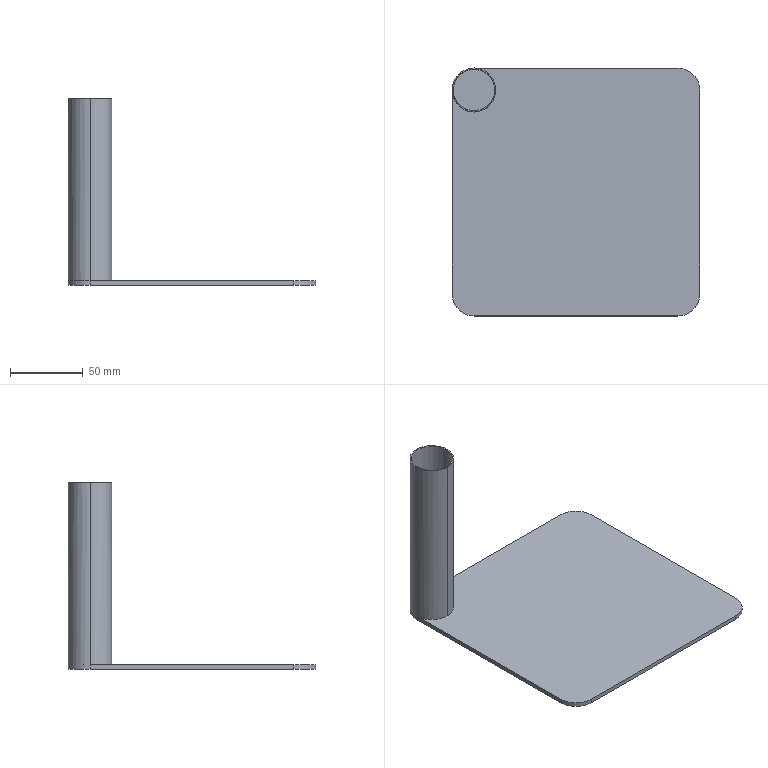Part | STEP file | Component1_1 | 1 solid | 15 faces | box 170 x 170 x 128 mm | volume 94175 mm3 | plane 8 | cylinder 7 | commonest cylinder face diameters 30 x5 28.6 x2
STEP:
#1=CARTESIAN_POINT('',(29.3,155.,2.));
#2=VERTEX_POINT('',#1);
#3=CARTESIAN_POINT('',(0.7,155.,2.));
#4=VERTEX_POINT('',#3);
#5=CARTESIAN_POINT('',(15.,155.,2.));
#6=DIRECTION('',(0.,0.,1.));
#7=DIRECTION('',(-1.,0.,0.));
#8=AXIS2_PLACEMENT_3D('',#5,#6,#7);
#9=CIRCLE('',#8,14.3);
#10=EDGE_CURVE('',#2,#4,#9,.T.);
#11=ORIENTED_EDGE('',*,*,#10,.F.);
#12=CARTESIAN_POINT('',(29.3,155.,127.));
#13=VERTEX_POINT('',#12);
#14=CARTESIAN_POINT('',(29.3,155.,2.));
#15=DIRECTION('',(0.,0.,1.));
#16=VECTOR('',#15,1000.);
#17=LINE('',#14,#16);
#18=EDGE_CURVE('',#2,#13,#17,.T.);
#19=ORIENTED_EDGE('',*,*,#18,.T.);
#20=CARTESIAN_POINT('',(0.7,155.,127.));
#21=VERTEX_POINT('',#20);
#22=CARTESIAN_POINT('',(15.,155.,127.));
#23=DIRECTION('',(0.,0.,-1.));
#24=DIRECTION('',(-1.,0.,0.));
#25=AXIS2_PLACEMENT_3D('',#22,#23,#24);
#26=CIRCLE('',#25,14.3);
#27=EDGE_CURVE('',#21,#13,#26,.T.);
#28=ORIENTED_EDGE('',*,*,#27,.F.);
#29=CARTESIAN_POINT('',(0.7,155.,2.));
#30=DIRECTION('',(0.,0.,1.));
#31=VECTOR('',#30,1000.);
#32=LINE('',#29,#31);
#33=EDGE_CURVE('',#4,#21,#32,.T.);
#34=ORIENTED_EDGE('',*,*,#33,.F.);
#35=EDGE_LOOP('',(#11,#19,#28,#34));
#36=FACE_OUTER_BOUND('',#35,.T.);
#37=CARTESIAN_POINT('',(15.,155.,2.));
#38=DIRECTION('',(0.,0.,1.));
#39=DIRECTION('',(-1.,0.,0.));
#40=AXIS2_PLACEMENT_3D('',#37,#38,#39);
#41=CYLINDRICAL_SURFACE('',#40,14.3);
#42=ADVANCED_FACE('',(#36),#41,.F.);
#43=CARTESIAN_POINT('',(15.,140.,2.));
#44=VERTEX_POINT('',#43);
#45=CARTESIAN_POINT('',(0.,155.,2.));
#46=VERTEX_POINT('',#45);
#47=CARTESIAN_POINT('',(15.,155.,2.));
#48=DIRECTION('',(0.,0.,-1.));
#49=DIRECTION('',(-1.,0.,0.));
#50=AXIS2_PLACEMENT_3D('',#47,#48,#49);
#51=CIRCLE('',#50,15.);
#52=EDGE_CURVE('',#44,#46,#51,.T.);
#53=ORIENTED_EDGE('',*,*,#52,.F.);
#54=CARTESIAN_POINT('',(15.,140.,127.));
#55=VERTEX_POINT('',#54);
#56=CARTESIAN_POINT('',(15.,140.,0.));
#57=DIRECTION('',(0.,0.,1.));
#58=VECTOR('',#57,1000.);
#59=LINE('',#56,#58);
#60=EDGE_CURVE('',#44,#55,#59,.T.);
#61=ORIENTED_EDGE('',*,*,#60,.T.);
#62=CARTESIAN_POINT('',(15.,170.,127.));
#63=VERTEX_POINT('',#62);
#64=CARTESIAN_POINT('',(15.,155.,127.));
#65=DIRECTION('',(0.,0.,1.));
#66=DIRECTION('',(-1.,0.,0.));
#67=AXIS2_PLACEMENT_3D('',#64,#65,#66);
#68=CIRCLE('',#67,15.);
#69=EDGE_CURVE('',#63,#55,#68,.T.);
#70=ORIENTED_EDGE('',*,*,#69,.F.);
#71=CARTESIAN_POINT('',(15.,170.,2.));
#72=VERTEX_POINT('',#71);
#73=CARTESIAN_POINT('',(15.,170.,0.));
#74=DIRECTION('',(0.,0.,1.));
#75=VECTOR('',#74,1000.);
#76=LINE('',#73,#75);
#77=EDGE_CURVE('',#72,#63,#76,.T.);
#78=ORIENTED_EDGE('',*,*,#77,.F.);
#79=CARTESIAN_POINT('',(15.,170.,-1.));
#80=VERTEX_POINT('',#79);
#81=CARTESIAN_POINT('',(15.,170.,0.));
#82=DIRECTION('',(0.,0.,-1.));
#83=VECTOR('',#82,1000.);
#84=LINE('',#81,#83);
#85=EDGE_CURVE('',#72,#80,#84,.T.);
#86=ORIENTED_EDGE('',*,*,#85,.T.);
#87=CARTESIAN_POINT('',(0.,155.,-1.));
#88=VERTEX_POINT('',#87);
#89=CARTESIAN_POINT('',(15.,155.,-1.));
#90=DIRECTION('',(0.,0.,-1.));
#91=DIRECTION('',(0.,1.,0.));
#92=AXIS2_PLACEMENT_3D('',#89,#90,#91);
#93=CIRCLE('',#92,15.);
#94=EDGE_CURVE('',#88,#80,#93,.T.);
#95=ORIENTED_EDGE('',*,*,#94,.F.);
#96=CARTESIAN_POINT('',(0.,155.,0.));
#97=DIRECTION('',(0.,0.,1.));
#98=VECTOR('',#97,1000.);
#99=LINE('',#96,#98);
#100=EDGE_CURVE('',#88,#46,#99,.T.);
#101=ORIENTED_EDGE('',*,*,#100,.T.);
#102=EDGE_LOOP('',(#53,#61,#70,#78,#86,#95,#101));
#103=FACE_OUTER_BOUND('',#102,.T.);
#104=CARTESIAN_POINT('',(15.,155.,0.));
#105=DIRECTION('',(0.,0.,1.));
#106=DIRECTION('',(0.,1.,0.));
#107=AXIS2_PLACEMENT_3D('',#104,#105,#106);
#108=CYLINDRICAL_SURFACE('',#107,15.);
#109=ADVANCED_FACE('',(#103),#108,.T.);
#110=CARTESIAN_POINT('',(15.,155.,2.));
#111=DIRECTION('',(0.,0.,1.));
#112=DIRECTION('',(-1.,0.,0.));
#113=AXIS2_PLACEMENT_3D('',#110,#111,#112);
#114=CIRCLE('',#113,14.3);
#115=EDGE_CURVE('',#4,#2,#114,.T.);
#116=ORIENTED_EDGE('',*,*,#115,.T.);
#117=ORIENTED_EDGE('',*,*,#10,.T.);
#118=EDGE_LOOP('',(#116,#117));
#119=FACE_OUTER_BOUND('',#118,.T.);
#120=CARTESIAN_POINT('',(85.,85.,2.));
#121=DIRECTION('',(0.,0.,1.));
#122=DIRECTION('',(1.,0.,0.));
#123=AXIS2_PLACEMENT_3D('',#120,#121,#122);
#124=PLANE('',#123);
#125=ADVANCED_FACE('',(#119),#124,.T.);
#126=ORIENTED_EDGE('',*,*,#60,.F.);
#127=CARTESIAN_POINT('',(15.,155.,2.));
#128=DIRECTION('',(0.,0.,-1.));
#129=DIRECTION('',(-1.,0.,0.));
#130=AXIS2_PLACEMENT_3D('',#127,#128,#129);
#131=CIRCLE('',#130,15.);
#132=EDGE_CURVE('',#72,#44,#131,.T.);
#133=ORIENTED_EDGE('',*,*,#132,.F.);
#134=ORIENTED_EDGE('',*,*,#77,.T.);
#135=CARTESIAN_POINT('',(15.,155.,127.));
#136=DIRECTION('',(0.,0.,1.));
#137=DIRECTION('',(-1.,0.,0.));
#138=AXIS2_PLACEMENT_3D('',#135,#136,#137);
#139=CIRCLE('',#138,15.);
#140=EDGE_CURVE('',#55,#63,#139,.T.);
#141=ORIENTED_EDGE('',*,*,#140,.F.);
#142=EDGE_LOOP('',(#126,#133,#134,#141));
#143=FACE_OUTER_BOUND('',#142,.T.);
#144=CARTESIAN_POINT('',(15.,155.,0.));
#145=DIRECTION('',(0.,0.,1.));
#146=DIRECTION('',(0.,1.,0.));
#147=AXIS2_PLACEMENT_3D('',#144,#145,#146);
#148=CYLINDRICAL_SURFACE('',#147,15.);
#149=ADVANCED_FACE('',(#143),#148,.T.);
#150=CARTESIAN_POINT('',(0.,15.,-1.));
#151=VERTEX_POINT('',#150);
#152=CARTESIAN_POINT('',(0.,15.,2.));
#153=VERTEX_POINT('',#152);
#154=CARTESIAN_POINT('',(0.,15.,0.));
#155=DIRECTION('',(0.,0.,1.));
#156=VECTOR('',#155,1000.);
#157=LINE('',#154,#156);
#158=EDGE_CURVE('',#151,#153,#157,.T.);
#159=ORIENTED_EDGE('',*,*,#158,.T.);
#160=CARTESIAN_POINT('',(0.,155.,2.));
#161=DIRECTION('',(0.,-1.,0.));
#162=VECTOR('',#161,1000.);
#163=LINE('',#160,#162);
#164=EDGE_CURVE('',#46,#153,#163,.T.);
#165=ORIENTED_EDGE('',*,*,#164,.F.);
#166=ORIENTED_EDGE('',*,*,#100,.F.);
#167=CARTESIAN_POINT('',(0.,155.,-1.));
#168=DIRECTION('',(0.,1.,0.));
#169=VECTOR('',#168,1000.);
#170=LINE('',#167,#169);
#171=EDGE_CURVE('',#151,#88,#170,.T.);
#172=ORIENTED_EDGE('',*,*,#171,.F.);
#173=EDGE_LOOP('',(#159,#165,#166,#172));
#174=FACE_OUTER_BOUND('',#173,.T.);
#175=CARTESIAN_POINT('',(0.,155.,0.));
#176=DIRECTION('',(-1.,0.,0.));
#177=DIRECTION('',(0.,1.,0.));
#178=AXIS2_PLACEMENT_3D('',#175,#176,#177);
#179=PLANE('',#178);
#180=ADVANCED_FACE('',(#174),#179,.T.);
#181=CARTESIAN_POINT('',(15.,0.,-1.));
#182=VERTEX_POINT('',#181);
#183=CARTESIAN_POINT('',(15.,0.,2.));
#184=VERTEX_POINT('',#183);
#185=CARTESIAN_POINT('',(15.,0.,0.));
#186=DIRECTION('',(0.,0.,1.));
#187=VECTOR('',#186,1000.);
#188=LINE('',#185,#187);
#189=EDGE_CURVE('',#182,#184,#188,.T.);
#190=ORIENTED_EDGE('',*,*,#189,.T.);
#191=CARTESIAN_POINT('',(15.,15.,2.));
#192=DIRECTION('',(0.,0.,1.));
#193=DIRECTION('',(-1.,0.,0.));
#194=AXIS2_PLACEMENT_3D('',#191,#192,#193);
#195=CIRCLE('',#194,15.);
#196=EDGE_CURVE('',#153,#184,#195,.T.);
#197=ORIENTED_EDGE('',*,*,#196,.F.);
#198=ORIENTED_EDGE('',*,*,#158,.F.);
#199=CARTESIAN_POINT('',(15.,15.,-1.));
#200=DIRECTION('',(0.,0.,-1.));
#201=DIRECTION('',(-1.,0.,0.));
#202=AXIS2_PLACEMENT_3D('',#199,#200,#201);
#203=CIRCLE('',#202,15.);
#204=EDGE_CURVE('',#182,#151,#203,.T.);
#205=ORIENTED_EDGE('',*,*,#204,.F.);
#206=EDGE_LOOP('',(#190,#197,#198,#205));
#207=FACE_OUTER_BOUND('',#206,.T.);
#208=CARTESIAN_POINT('',(15.,15.,0.));
#209=DIRECTION('',(0.,0.,1.));
#210=DIRECTION('',(-1.,0.,0.));
#211=AXIS2_PLACEMENT_3D('',#208,#209,#210);
#212=CYLINDRICAL_SURFACE('',#211,15.);
#213=ADVANCED_FACE('',(#207),#212,.T.);
#214=CARTESIAN_POINT('',(155.,0.,-1.));
#215=VERTEX_POINT('',#214);
#216=CARTESIAN_POINT('',(155.,0.,2.));
#217=VERTEX_POINT('',#216);
#218=CARTESIAN_POINT('',(155.,0.,0.));
#219=DIRECTION('',(0.,0.,1.));
#220=VECTOR('',#219,1000.);
#221=LINE('',#218,#220);
#222=EDGE_CURVE('',#215,#217,#221,.T.);
#223=ORIENTED_EDGE('',*,*,#222,.T.);
#224=CARTESIAN_POINT('',(15.,0.,2.));
#225=DIRECTION('',(1.,0.,0.));
#226=VECTOR('',#225,1000.);
#227=LINE('',#224,#226);
#228=EDGE_CURVE('',#184,#217,#227,.T.);
#229=ORIENTED_EDGE('',*,*,#228,.F.);
#230=ORIENTED_EDGE('',*,*,#189,.F.);
#231=CARTESIAN_POINT('',(15.,0.,-1.));
#232=DIRECTION('',(-1.,0.,0.));
#233=VECTOR('',#232,1000.);
#234=LINE('',#231,#233);
#235=EDGE_CURVE('',#215,#182,#234,.T.);
#236=ORIENTED_EDGE('',*,*,#235,.F.);
#237=EDGE_LOOP('',(#223,#229,#230,#236));
#238=FACE_OUTER_BOUND('',#237,.T.);
#239=CARTESIAN_POINT('',(15.,0.,0.));
#240=DIRECTION('',(0.,-1.,0.));
#241=DIRECTION('',(0.,0.,-1.));
#242=AXIS2_PLACEMENT_3D('',#239,#240,#241);
#243=PLANE('',#242);
#244=ADVANCED_FACE('',(#238),#243,.T.);
#245=CARTESIAN_POINT('',(170.,15.,-1.));
#246=VERTEX_POINT('',#245);
#247=CARTESIAN_POINT('',(170.,15.,2.));
#248=VERTEX_POINT('',#247);
#249=CARTESIAN_POINT('',(170.,15.,0.));
#250=DIRECTION('',(0.,0.,1.));
#251=VECTOR('',#250,1000.);
#252=LINE('',#249,#251);
#253=EDGE_CURVE('',#246,#248,#252,.T.);
#254=ORIENTED_EDGE('',*,*,#253,.T.);
#255=CARTESIAN_POINT('',(155.,15.,2.));
#256=DIRECTION('',(0.,0.,1.));
#257=DIRECTION('',(0.,-1.,0.));
#258=AXIS2_PLACEMENT_3D('',#255,#256,#257);
#259=CIRCLE('',#258,15.);
#260=EDGE_CURVE('',#217,#248,#259,.T.);
#261=ORIENTED_EDGE('',*,*,#260,.F.);
#262=ORIENTED_EDGE('',*,*,#222,.F.);
#263=CARTESIAN_POINT('',(155.,15.,-1.));
#264=DIRECTION('',(0.,0.,-1.));
#265=DIRECTION('',(0.,-1.,0.));
#266=AXIS2_PLACEMENT_3D('',#263,#264,#265);
#267=CIRCLE('',#266,15.);
#268=EDGE_CURVE('',#246,#215,#267,.T.);
#269=ORIENTED_EDGE('',*,*,#268,.F.);
#270=EDGE_LOOP('',(#254,#261,#262,#269));
#271=FACE_OUTER_BOUND('',#270,.T.);
#272=CARTESIAN_POINT('',(155.,15.,0.));
#273=DIRECTION('',(0.,0.,1.));
#274=DIRECTION('',(0.,-1.,0.));
#275=AXIS2_PLACEMENT_3D('',#272,#273,#274);
#276=CYLINDRICAL_SURFACE('',#275,15.);
#277=ADVANCED_FACE('',(#271),#276,.T.);
#278=CARTESIAN_POINT('',(170.,155.,-1.));
#279=VERTEX_POINT('',#278);
#280=CARTESIAN_POINT('',(170.,155.,2.));
#281=VERTEX_POINT('',#280);
#282=CARTESIAN_POINT('',(170.,155.,0.));
#283=DIRECTION('',(0.,0.,1.));
#284=VECTOR('',#283,1000.);
#285=LINE('',#282,#284);
#286=EDGE_CURVE('',#279,#281,#285,.T.);
#287=ORIENTED_EDGE('',*,*,#286,.T.);
#288=CARTESIAN_POINT('',(170.,15.,2.));
#289=DIRECTION('',(0.,1.,0.));
#290=VECTOR('',#289,1000.);
#291=LINE('',#288,#290);
#292=EDGE_CURVE('',#248,#281,#291,.T.);
#293=ORIENTED_EDGE('',*,*,#292,.F.);
#294=ORIENTED_EDGE('',*,*,#253,.F.);
#295=CARTESIAN_POINT('',(170.,15.,-1.));
#296=DIRECTION('',(0.,-1.,0.));
#297=VECTOR('',#296,1000.);
#298=LINE('',#295,#297);
#299=EDGE_CURVE('',#279,#246,#298,.T.);
#300=ORIENTED_EDGE('',*,*,#299,.F.);
#301=EDGE_LOOP('',(#287,#293,#294,#300));
#302=FACE_OUTER_BOUND('',#301,.T.);
#303=CARTESIAN_POINT('',(170.,15.,0.));
#304=DIRECTION('',(1.,0.,0.));
#305=DIRECTION('',(0.,1.,0.));
#306=AXIS2_PLACEMENT_3D('',#303,#304,#305);
#307=PLANE('',#306);
#308=ADVANCED_FACE('',(#302),#307,.T.);
#309=CARTESIAN_POINT('',(155.,170.,-1.));
#310=VERTEX_POINT('',#309);
#311=CARTESIAN_POINT('',(155.,170.,2.));
#312=VERTEX_POINT('',#311);
#313=CARTESIAN_POINT('',(155.,170.,0.));
#314=DIRECTION('',(0.,0.,1.));
#315=VECTOR('',#314,1000.);
#316=LINE('',#313,#315);
#317=EDGE_CURVE('',#310,#312,#316,.T.);
#318=ORIENTED_EDGE('',*,*,#317,.T.);
#319=CARTESIAN_POINT('',(155.,155.,2.));
#320=DIRECTION('',(0.,0.,1.));
#321=DIRECTION('',(1.,0.,0.));
#322=AXIS2_PLACEMENT_3D('',#319,#320,#321);
#323=CIRCLE('',#322,15.);
#324=EDGE_CURVE('',#281,#312,#323,.T.);
#325=ORIENTED_EDGE('',*,*,#324,.F.);
#326=ORIENTED_EDGE('',*,*,#286,.F.);
#327=CARTESIAN_POINT('',(155.,155.,-1.));
#328=DIRECTION('',(0.,0.,-1.));
#329=DIRECTION('',(1.,0.,0.));
#330=AXIS2_PLACEMENT_3D('',#327,#328,#329);
#331=CIRCLE('',#330,15.);
#332=EDGE_CURVE('',#310,#279,#331,.T.);
#333=ORIENTED_EDGE('',*,*,#332,.F.);
#334=EDGE_LOOP('',(#318,#325,#326,#333));
#335=FACE_OUTER_BOUND('',#334,.T.);
#336=CARTESIAN_POINT('',(155.,155.,0.));
#337=DIRECTION('',(0.,0.,1.));
#338=DIRECTION('',(1.,0.,0.));
#339=AXIS2_PLACEMENT_3D('',#336,#337,#338);
#340=CYLINDRICAL_SURFACE('',#339,15.);
#341=ADVANCED_FACE('',(#335),#340,.T.);
#342=ORIENTED_EDGE('',*,*,#85,.F.);
#343=CARTESIAN_POINT('',(155.,170.,2.));
#344=DIRECTION('',(-1.,0.,0.));
#345=VECTOR('',#344,1000.);
#346=LINE('',#343,#345);
#347=EDGE_CURVE('',#312,#72,#346,.T.);
#348=ORIENTED_EDGE('',*,*,#347,.F.);
#349=ORIENTED_EDGE('',*,*,#317,.F.);
#350=CARTESIAN_POINT('',(155.,170.,-1.));
#351=DIRECTION('',(1.,0.,0.));
#352=VECTOR('',#351,1000.);
#353=LINE('',#350,#352);
#354=EDGE_CURVE('',#80,#310,#353,.T.);
#355=ORIENTED_EDGE('',*,*,#354,.F.);
#356=EDGE_LOOP('',(#342,#348,#349,#355));
#357=FACE_OUTER_BOUND('',#356,.T.);
#358=CARTESIAN_POINT('',(155.,170.,0.));
#359=DIRECTION('',(0.,1.,0.));
#360=DIRECTION('',(1.,0.,0.));
#361=AXIS2_PLACEMENT_3D('',#358,#359,#360);
#362=PLANE('',#361);
#363=ADVANCED_FACE('',(#357),#362,.T.);
#364=ORIENTED_EDGE('',*,*,#132,.T.);
#365=ORIENTED_EDGE('',*,*,#52,.T.);
#366=ORIENTED_EDGE('',*,*,#164,.T.);
#367=ORIENTED_EDGE('',*,*,#196,.T.);
#368=ORIENTED_EDGE('',*,*,#228,.T.);
#369=ORIENTED_EDGE('',*,*,#260,.T.);
#370=ORIENTED_EDGE('',*,*,#292,.T.);
#371=ORIENTED_EDGE('',*,*,#324,.T.);
#372=ORIENTED_EDGE('',*,*,#347,.T.);
#373=EDGE_LOOP('',(#364,#365,#366,#367,#368,#369,#370,#371,#372));
#374=FACE_OUTER_BOUND('',#373,.T.);
#375=CARTESIAN_POINT('',(85.,85.,2.));
#376=DIRECTION('',(0.,0.,1.));
#377=DIRECTION('',(1.,0.,0.));
#378=AXIS2_PLACEMENT_3D('',#375,#376,#377);
#379=PLANE('',#378);
#380=ADVANCED_FACE('',(#374),#379,.T.);
#381=ORIENTED_EDGE('',*,*,#27,.T.);
#382=CARTESIAN_POINT('',(15.,155.,127.));
#383=DIRECTION('',(0.,0.,-1.));
#384=DIRECTION('',(-1.,0.,0.));
#385=AXIS2_PLACEMENT_3D('',#382,#383,#384);
#386=CIRCLE('',#385,14.3);
#387=EDGE_CURVE('',#13,#21,#386,.T.);
#388=ORIENTED_EDGE('',*,*,#387,.T.);
#389=EDGE_LOOP('',(#381,#388));
#390=FACE_BOUND('',#389,.T.);
#391=ORIENTED_EDGE('',*,*,#69,.T.);
#392=ORIENTED_EDGE('',*,*,#140,.T.);
#393=EDGE_LOOP('',(#391,#392));
#394=FACE_OUTER_BOUND('',#393,.T.);
#395=CARTESIAN_POINT('',(15.,155.,127.));
#396=DIRECTION('',(0.,0.,1.));
#397=DIRECTION('',(1.,0.,0.));
#398=AXIS2_PLACEMENT_3D('',#395,#396,#397);
#399=PLANE('',#398);
#400=ADVANCED_FACE('',(#390,#394),#399,.T.);
#401=ORIENTED_EDGE('',*,*,#18,.F.);
#402=ORIENTED_EDGE('',*,*,#115,.F.);
#403=ORIENTED_EDGE('',*,*,#33,.T.);
#404=ORIENTED_EDGE('',*,*,#387,.F.);
#405=EDGE_LOOP('',(#401,#402,#403,#404));
#406=FACE_OUTER_BOUND('',#405,.T.);
#407=CARTESIAN_POINT('',(15.,155.,2.));
#408=DIRECTION('',(0.,0.,1.));
#409=DIRECTION('',(-1.,0.,0.));
#410=AXIS2_PLACEMENT_3D('',#407,#408,#409);
#411=CYLINDRICAL_SURFACE('',#410,14.3);
#412=ADVANCED_FACE('',(#406),#411,.F.);
#413=ORIENTED_EDGE('',*,*,#94,.T.);
#414=ORIENTED_EDGE('',*,*,#354,.T.);
#415=ORIENTED_EDGE('',*,*,#332,.T.);
#416=ORIENTED_EDGE('',*,*,#299,.T.);
#417=ORIENTED_EDGE('',*,*,#268,.T.);
#418=ORIENTED_EDGE('',*,*,#235,.T.);
#419=ORIENTED_EDGE('',*,*,#204,.T.);
#420=ORIENTED_EDGE('',*,*,#171,.T.);
#421=EDGE_LOOP('',(#413,#414,#415,#416,#417,#418,#419,#420));
#422=FACE_OUTER_BOUND('',#421,.T.);
#423=CARTESIAN_POINT('',(85.,85.,-1.));
#424=DIRECTION('',(0.,0.,1.));
#425=DIRECTION('',(1.,0.,0.));
#426=AXIS2_PLACEMENT_3D('',#423,#424,#425);
#427=PLANE('',#426);
#428=ADVANCED_FACE('',(#422),#427,.F.);
#429=CLOSED_SHELL('',(#42,#109,#125,#149,#180,#213,#244,#277,#308,#341,#363,#380,#400,#412,#428));
#430=MANIFOLD_SOLID_BREP('',#429);
#431=CARTESIAN_POINT('',(0.,0.,0.));
#432=DIRECTION('',(0.,0.,1.));
#433=DIRECTION('',(1.,0.,0.));
#434=AXIS2_PLACEMENT_3D('',#431,#432,#433);
#435=(LENGTH_UNIT()NAMED_UNIT(*)SI_UNIT(.MILLI.,.METRE.));
#436=UNCERTAINTY_MEASURE_WITH_UNIT(LENGTH_MEASURE(0.00001),#435,'','');
#437=(NAMED_UNIT(*)PLANE_ANGLE_UNIT()SI_UNIT($,.RADIAN.));
#438=(NAMED_UNIT(*)SI_UNIT($,.STERADIAN.)SOLID_ANGLE_UNIT());
#439=(GEOMETRIC_REPRESENTATION_CONTEXT(3)GLOBAL_UNCERTAINTY_ASSIGNED_CONTEXT((#436))GLOBAL_UNIT_ASSIGNED_CONTEXT((#435,#437,#438))REPRESENTATION_CONTEXT('',''));
#440=ADVANCED_BREP_SHAPE_REPRESENTATION('',(#430,#434),#439);